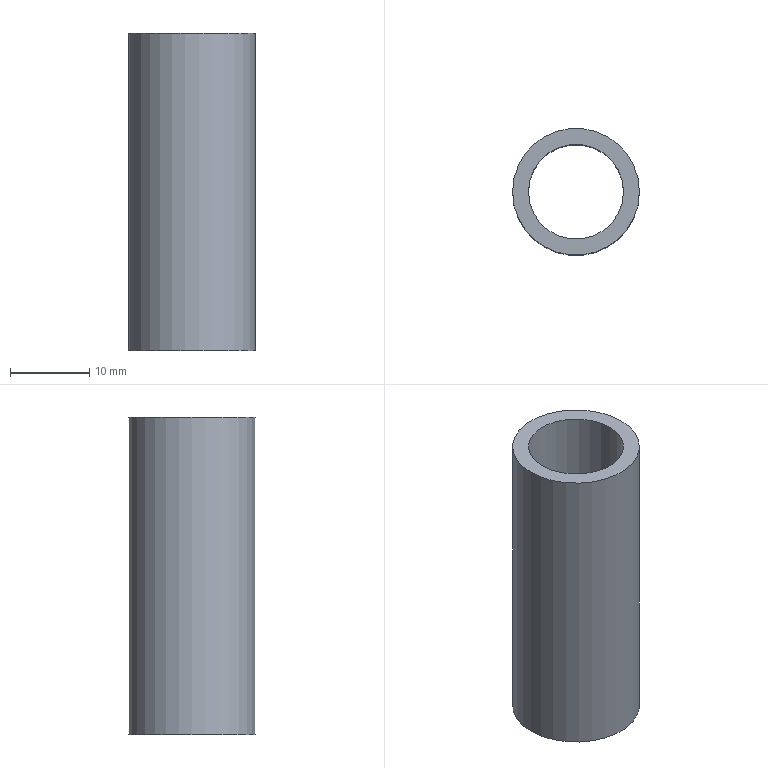Part | NX | features solid 2 | 1 solid | 4 faces | box 16 x 16 x 40 mm | volume 3519 mm3 | plane 2 | cylinder 2 | commonest cylinder face diameters 12 x1 16 x1
STEP:
#1=CARTESIAN_POINT('',(-1166.,380.,3.));
#2=VERTEX_POINT('',#1);
#3=CARTESIAN_POINT('',(-1160.,380.,3.));
#4=DIRECTION('',(0.,0.,-1.));
#5=DIRECTION('',(-1.,0.,0.));
#6=AXIS2_PLACEMENT_3D('',#3,#4,#5);
#7=CIRCLE('',#6,6.);
#8=EDGE_CURVE('',#2,#2,#7,.F.);
#9=ORIENTED_EDGE('',*,*,#8,.T.);
#10=EDGE_LOOP('',(#9));
#11=FACE_BOUND('',#10,.T.);
#12=CARTESIAN_POINT('',(-1168.,380.,3.));
#13=VERTEX_POINT('',#12);
#14=CARTESIAN_POINT('',(-1160.,380.,3.));
#15=DIRECTION('',(0.,0.,-1.));
#16=DIRECTION('',(-1.,0.,0.));
#17=AXIS2_PLACEMENT_3D('',#14,#15,#16);
#18=CIRCLE('',#17,8.);
#19=EDGE_CURVE('',#13,#13,#18,.F.);
#20=ORIENTED_EDGE('',*,*,#19,.F.);
#21=EDGE_LOOP('',(#20));
#22=FACE_BOUND('',#21,.T.);
#23=CARTESIAN_POINT('',(-1208.358,435.,3.));
#24=DIRECTION('',(0.,0.,-1.));
#25=DIRECTION('',(-1.,0.,0.));
#26=AXIS2_PLACEMENT_3D('',#23,#24,#25);
#27=PLANE('',#26);
#28=ADVANCED_FACE('',(#11,#22),#27,.T.);
#29=CARTESIAN_POINT('',(-1166.,380.,43.));
#30=VERTEX_POINT('',#29);
#31=CARTESIAN_POINT('',(-1160.,380.,43.));
#32=DIRECTION('',(0.,0.,-1.));
#33=DIRECTION('',(-1.,0.,0.));
#34=AXIS2_PLACEMENT_3D('',#31,#32,#33);
#35=CIRCLE('',#34,6.);
#36=EDGE_CURVE('',#30,#30,#35,.F.);
#37=ORIENTED_EDGE('',*,*,#36,.F.);
#38=EDGE_LOOP('',(#37));
#39=FACE_BOUND('',#38,.T.);
#40=CARTESIAN_POINT('',(-1152.,380.,43.));
#41=VERTEX_POINT('',#40);
#42=CARTESIAN_POINT('',(-1160.,380.,43.));
#43=DIRECTION('',(0.,0.,1.));
#44=DIRECTION('',(1.,0.,0.));
#45=AXIS2_PLACEMENT_3D('',#42,#43,#44);
#46=CIRCLE('',#45,8.);
#47=EDGE_CURVE('',#41,#41,#46,.T.);
#48=ORIENTED_EDGE('',*,*,#47,.T.);
#49=EDGE_LOOP('',(#48));
#50=FACE_BOUND('',#49,.T.);
#51=CARTESIAN_POINT('',(-1160.,380.,43.));
#52=DIRECTION('',(0.,0.,-1.));
#53=DIRECTION('',(-1.,0.,0.));
#54=AXIS2_PLACEMENT_3D('',#51,#52,#53);
#55=PLANE('',#54);
#56=ADVANCED_FACE('',(#39,#50),#55,.F.);
#57=ORIENTED_EDGE('',*,*,#8,.F.);
#58=EDGE_LOOP('',(#57));
#59=FACE_BOUND('',#58,.T.);
#60=ORIENTED_EDGE('',*,*,#36,.T.);
#61=EDGE_LOOP('',(#60));
#62=FACE_BOUND('',#61,.T.);
#63=CARTESIAN_POINT('',(-1160.,380.,43.));
#64=DIRECTION('',(0.,0.,-1.));
#65=DIRECTION('',(-1.,0.,0.));
#66=AXIS2_PLACEMENT_3D('',#63,#64,#65);
#67=CYLINDRICAL_SURFACE('',#66,6.);
#68=ADVANCED_FACE('',(#59,#62),#67,.F.);
#69=ORIENTED_EDGE('',*,*,#19,.T.);
#70=EDGE_LOOP('',(#69));
#71=FACE_BOUND('',#70,.T.);
#72=ORIENTED_EDGE('',*,*,#47,.F.);
#73=EDGE_LOOP('',(#72));
#74=FACE_BOUND('',#73,.T.);
#75=CARTESIAN_POINT('',(-1160.,380.,43.));
#76=DIRECTION('',(0.,0.,-1.));
#77=DIRECTION('',(-1.,0.,0.));
#78=AXIS2_PLACEMENT_3D('',#75,#76,#77);
#79=CYLINDRICAL_SURFACE('',#78,8.);
#80=ADVANCED_FACE('',(#71,#74),#79,.T.);
#81=CLOSED_SHELL('',(#28,#56,#68,#80));
#82=MANIFOLD_SOLID_BREP('',#81);
#83=(LENGTH_UNIT()NAMED_UNIT(*)SI_UNIT(.MILLI.,.METRE.));
#84=UNCERTAINTY_MEASURE_WITH_UNIT(LENGTH_MEASURE(0.00001),#83,'','');
#85=(NAMED_UNIT(*)PLANE_ANGLE_UNIT()SI_UNIT($,.RADIAN.));
#86=(NAMED_UNIT(*)SI_UNIT($,.STERADIAN.)SOLID_ANGLE_UNIT());
#87=(GEOMETRIC_REPRESENTATION_CONTEXT(3)GLOBAL_UNCERTAINTY_ASSIGNED_CONTEXT((#84))GLOBAL_UNIT_ASSIGNED_CONTEXT((#83,#85,#86))REPRESENTATION_CONTEXT('',''));
#88=ADVANCED_BREP_SHAPE_REPRESENTATION('',(#82),#87);